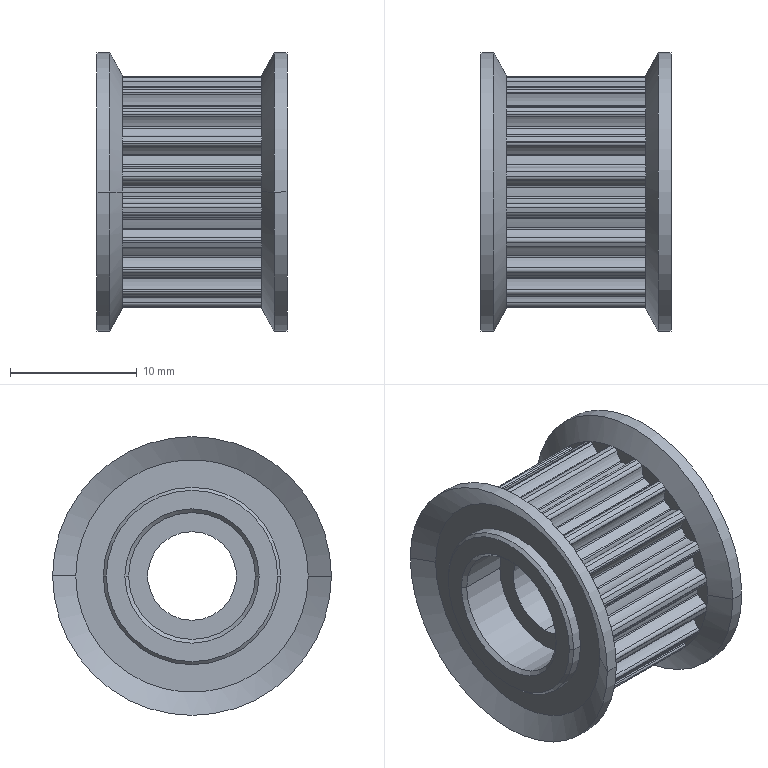Part | SolidWorks | features BaseBody 1 | 1 solid | 257 faces | box 15 x 22 x 22 mm | volume 2686 mm3 | cylinder 195 | plane 46 | cone 16 | commonest cylinder face diameters 0.56 x54 0.3 x44 3.95 x42 16.12 x21 18.34 x20 10 x4